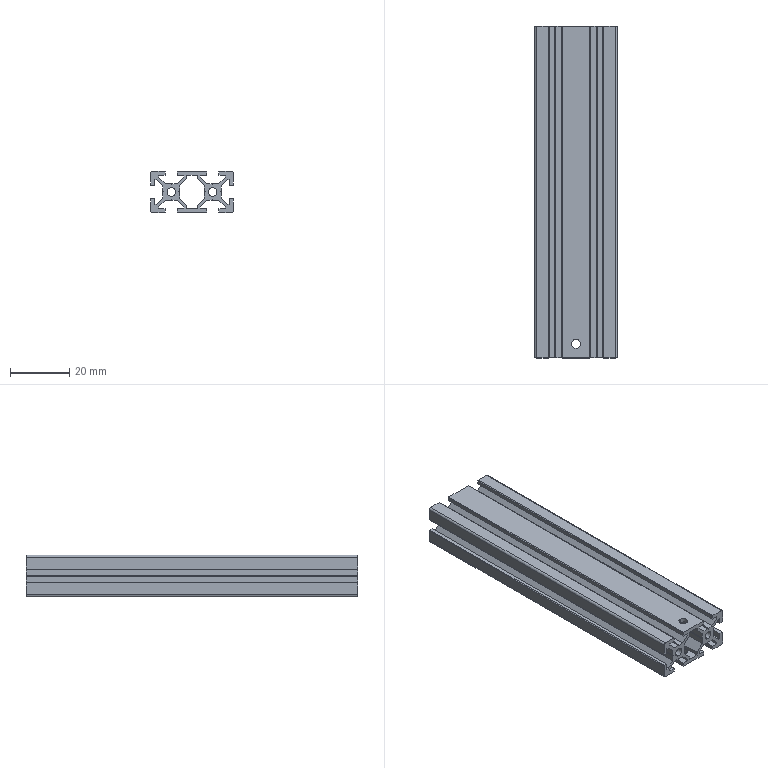Part | SolidWorks | features SplitBody 1 | 1 solid | 126 faces | box 28 x 112 x 14 mm | volume 17740 mm3 | plane 102 | cylinder 24 | commonest cylinder face diameters 0.42 x12 1.4 x4 2.8 x4 3 x4